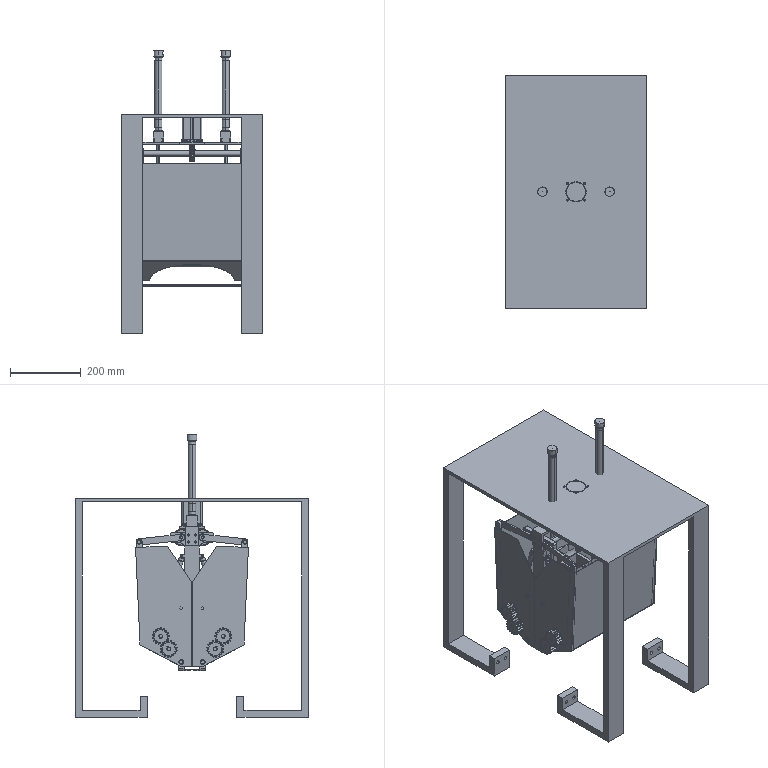Part | SolidWorks | 209 solids | 3860 faces | volume 9842736 mm3 | cylinder 1365 | plane 924 | spline 588 | cone 501 | torus 290 | sphere 192 | commonest cylinder face diameters 45.739 x128 10 x122 6 x104 12 x82 36.25 x68 47.5 x68